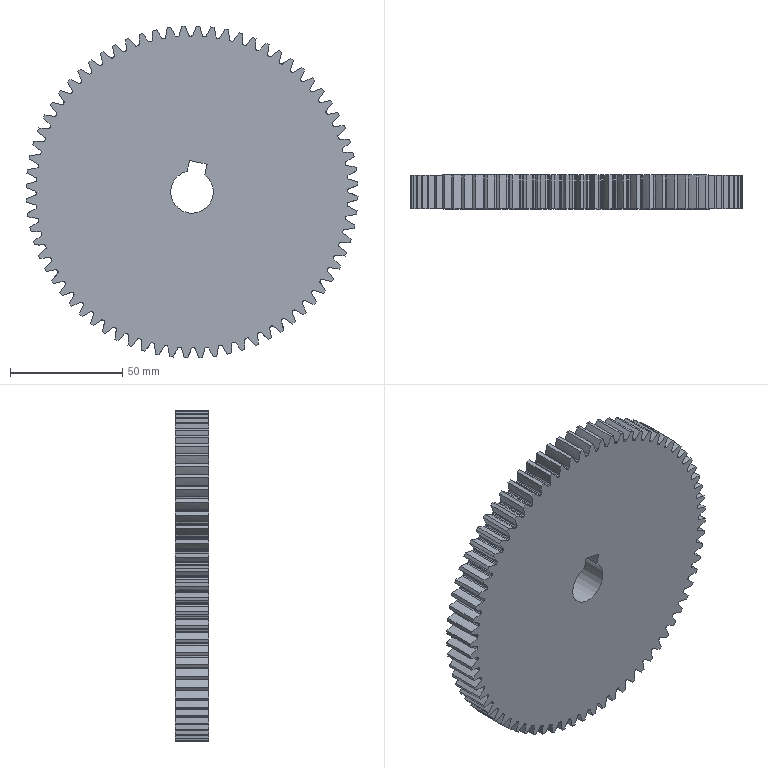Part | STEP file | 1_BODY_id910_x_t | 1 solid | 438 faces | box 147.953 x 15 x 147.953 mm | volume 238621 mm3 | other 360 | cylinder 73 | plane 5 | commonest cylinder face diameters 139 x72 19 x1